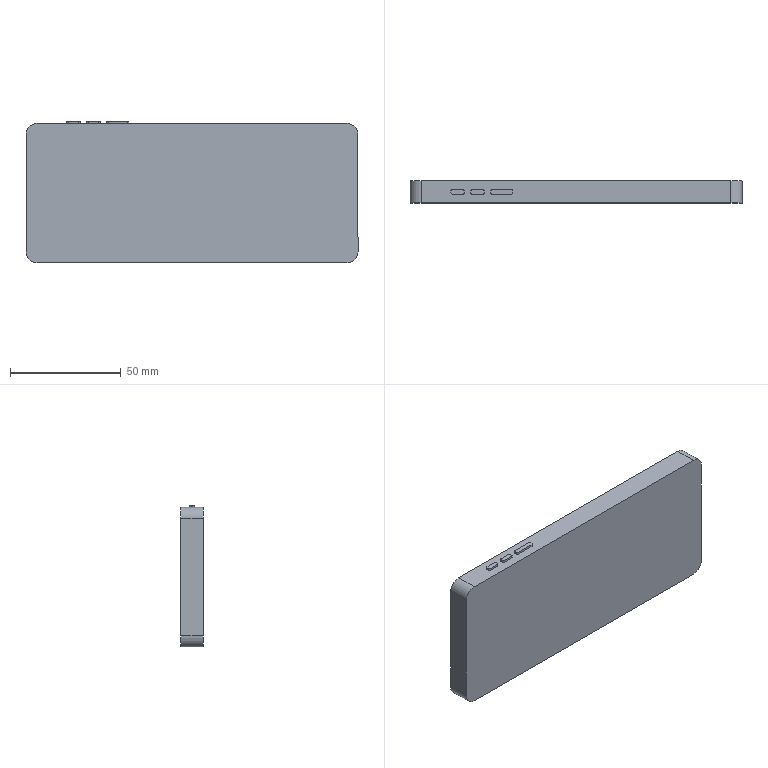Part | NX | features DATUM_CSYS 3, BLEND 2, EXTRUDE 2, SKETCH 2 | 1 solid | 37 faces | box 150 x 10 x 64.04 mm | volume 94388 mm3 | plane 21 | cylinder 16 | commonest cylinder face diameters 1.2 x12 10 x4
STEP:
#1=CARTESIAN_POINT('',(-47.486,-4.6,31.52));
#2=VERTEX_POINT('',#1);
#3=CARTESIAN_POINT('',(-47.486,-5.4,31.52));
#4=VERTEX_POINT('',#3);
#5=CARTESIAN_POINT('',(-47.486,-4.,31.52));
#6=DIRECTION('',(0.,-1.,0.));
#7=VECTOR('',#6,1000.);
#8=LINE('',#5,#7);
#9=EDGE_CURVE('',#2,#4,#8,.T.);
#10=ORIENTED_EDGE('',*,*,#9,.F.);
#11=CARTESIAN_POINT('',(-46.886,-4.,31.52));
#12=VERTEX_POINT('',#11);
#13=CARTESIAN_POINT('',(-46.886,-4.6,31.52));
#14=DIRECTION('',(0.,0.,-1.));
#15=DIRECTION('',(-1.,0.,0.));
#16=AXIS2_PLACEMENT_3D('',#13,#14,#15);
#17=CIRCLE('',#16,0.6);
#18=EDGE_CURVE('',#2,#12,#17,.T.);
#19=ORIENTED_EDGE('',*,*,#18,.T.);
#20=CARTESIAN_POINT('',(-42.086,-4.,31.52));
#21=VERTEX_POINT('',#20);
#22=CARTESIAN_POINT('',(-41.486,-4.,31.52));
#23=DIRECTION('',(-1.,0.,0.));
#24=VECTOR('',#23,1000.);
#25=LINE('',#22,#24);
#26=EDGE_CURVE('',#21,#12,#25,.T.);
#27=ORIENTED_EDGE('',*,*,#26,.F.);
#28=CARTESIAN_POINT('',(-41.486,-4.6,31.52));
#29=VERTEX_POINT('',#28);
#30=CARTESIAN_POINT('',(-42.086,-4.6,31.52));
#31=DIRECTION('',(0.,0.,-1.));
#32=DIRECTION('',(-1.,0.,0.));
#33=AXIS2_PLACEMENT_3D('',#30,#31,#32);
#34=CIRCLE('',#33,0.6);
#35=EDGE_CURVE('',#21,#29,#34,.T.);
#36=ORIENTED_EDGE('',*,*,#35,.T.);
#37=CARTESIAN_POINT('',(-41.486,-5.4,31.52));
#38=VERTEX_POINT('',#37);
#39=CARTESIAN_POINT('',(-41.486,-6.,31.52));
#40=DIRECTION('',(0.,1.,0.));
#41=VECTOR('',#40,1000.);
#42=LINE('',#39,#41);
#43=EDGE_CURVE('',#38,#29,#42,.T.);
#44=ORIENTED_EDGE('',*,*,#43,.F.);
#45=CARTESIAN_POINT('',(-42.086,-6.,31.52));
#46=VERTEX_POINT('',#45);
#47=CARTESIAN_POINT('',(-42.086,-5.4,31.52));
#48=DIRECTION('',(0.,0.,-1.));
#49=DIRECTION('',(-1.,0.,0.));
#50=AXIS2_PLACEMENT_3D('',#47,#48,#49);
#51=CIRCLE('',#50,0.6);
#52=EDGE_CURVE('',#38,#46,#51,.T.);
#53=ORIENTED_EDGE('',*,*,#52,.T.);
#54=CARTESIAN_POINT('',(-46.886,-6.,31.52));
#55=VERTEX_POINT('',#54);
#56=CARTESIAN_POINT('',(-47.486,-6.,31.52));
#57=DIRECTION('',(1.,0.,0.));
#58=VECTOR('',#57,1000.);
#59=LINE('',#56,#58);
#60=EDGE_CURVE('',#55,#46,#59,.T.);
#61=ORIENTED_EDGE('',*,*,#60,.F.);
#62=CARTESIAN_POINT('',(-46.886,-5.4,31.52));
#63=DIRECTION('',(0.,0.,-1.));
#64=DIRECTION('',(-1.,0.,0.));
#65=AXIS2_PLACEMENT_3D('',#62,#63,#64);
#66=CIRCLE('',#65,0.6);
#67=EDGE_CURVE('',#55,#4,#66,.T.);
#68=ORIENTED_EDGE('',*,*,#67,.T.);
#69=EDGE_LOOP('',(#10,#19,#27,#36,#44,#53,#61,#68));
#70=FACE_BOUND('',#69,.T.);
#71=CARTESIAN_POINT('',(70.,0.,31.52));
#72=VERTEX_POINT('',#71);
#73=CARTESIAN_POINT('',(-70.,0.,31.52));
#74=VERTEX_POINT('',#73);
#75=CARTESIAN_POINT('',(75.,0.,31.52));
#76=DIRECTION('',(-1.,0.,0.));
#77=VECTOR('',#76,1000.);
#78=LINE('',#75,#77);
#79=EDGE_CURVE('',#72,#74,#78,.T.);
#80=ORIENTED_EDGE('',*,*,#79,.T.);
#81=CARTESIAN_POINT('',(-70.,-10.,31.52));
#82=VERTEX_POINT('',#81);
#83=CARTESIAN_POINT('',(-70.,-10.,31.52));
#84=DIRECTION('',(0.,1.,0.));
#85=VECTOR('',#84,1000.);
#86=LINE('',#83,#85);
#87=EDGE_CURVE('',#74,#82,#86,.F.);
#88=ORIENTED_EDGE('',*,*,#87,.T.);
#89=CARTESIAN_POINT('',(70.,-10.,31.52));
#90=VERTEX_POINT('',#89);
#91=CARTESIAN_POINT('',(75.,-10.,31.52));
#92=DIRECTION('',(-1.,0.,0.));
#93=VECTOR('',#92,1000.);
#94=LINE('',#91,#93);
#95=EDGE_CURVE('',#90,#82,#94,.T.);
#96=ORIENTED_EDGE('',*,*,#95,.F.);
#97=CARTESIAN_POINT('',(70.,-10.,31.52));
#98=DIRECTION('',(0.,1.,0.));
#99=VECTOR('',#98,1000.);
#100=LINE('',#97,#99);
#101=EDGE_CURVE('',#90,#72,#100,.T.);
#102=ORIENTED_EDGE('',*,*,#101,.T.);
#103=EDGE_LOOP('',(#80,#88,#96,#102));
#104=FACE_BOUND('',#103,.T.);
#105=CARTESIAN_POINT('',(-38.486,-4.6,31.52));
#106=VERTEX_POINT('',#105);
#107=CARTESIAN_POINT('',(-38.486,-5.4,31.52));
#108=VERTEX_POINT('',#107);
#109=CARTESIAN_POINT('',(-38.486,-4.,31.52));
#110=DIRECTION('',(0.,-1.,0.));
#111=VECTOR('',#110,1000.);
#112=LINE('',#109,#111);
#113=EDGE_CURVE('',#106,#108,#112,.T.);
#114=ORIENTED_EDGE('',*,*,#113,.F.);
#115=CARTESIAN_POINT('',(-37.886,-4.,31.52));
#116=VERTEX_POINT('',#115);
#117=CARTESIAN_POINT('',(-37.886,-4.6,31.52));
#118=DIRECTION('',(0.,0.,-1.));
#119=DIRECTION('',(-1.,0.,0.));
#120=AXIS2_PLACEMENT_3D('',#117,#118,#119);
#121=CIRCLE('',#120,0.6);
#122=EDGE_CURVE('',#106,#116,#121,.T.);
#123=ORIENTED_EDGE('',*,*,#122,.T.);
#124=CARTESIAN_POINT('',(-29.086,-4.,31.52));
#125=VERTEX_POINT('',#124);
#126=CARTESIAN_POINT('',(-28.486,-4.,31.52));
#127=DIRECTION('',(-1.,0.,0.));
#128=VECTOR('',#127,1000.);
#129=LINE('',#126,#128);
#130=EDGE_CURVE('',#125,#116,#129,.T.);
#131=ORIENTED_EDGE('',*,*,#130,.F.);
#132=CARTESIAN_POINT('',(-28.486,-4.6,31.52));
#133=VERTEX_POINT('',#132);
#134=CARTESIAN_POINT('',(-29.086,-4.6,31.52));
#135=DIRECTION('',(0.,0.,-1.));
#136=DIRECTION('',(-1.,0.,0.));
#137=AXIS2_PLACEMENT_3D('',#134,#135,#136);
#138=CIRCLE('',#137,0.6);
#139=EDGE_CURVE('',#125,#133,#138,.T.);
#140=ORIENTED_EDGE('',*,*,#139,.T.);
#141=CARTESIAN_POINT('',(-28.486,-5.4,31.52));
#142=VERTEX_POINT('',#141);
#143=CARTESIAN_POINT('',(-28.486,-6.,31.52));
#144=DIRECTION('',(0.,1.,0.));
#145=VECTOR('',#144,1000.);
#146=LINE('',#143,#145);
#147=EDGE_CURVE('',#142,#133,#146,.T.);
#148=ORIENTED_EDGE('',*,*,#147,.F.);
#149=CARTESIAN_POINT('',(-29.086,-6.,31.52));
#150=VERTEX_POINT('',#149);
#151=CARTESIAN_POINT('',(-29.086,-5.4,31.52));
#152=DIRECTION('',(0.,0.,-1.));
#153=DIRECTION('',(-1.,0.,0.));
#154=AXIS2_PLACEMENT_3D('',#151,#152,#153);
#155=CIRCLE('',#154,0.6);
#156=EDGE_CURVE('',#142,#150,#155,.T.);
#157=ORIENTED_EDGE('',*,*,#156,.T.);
#158=CARTESIAN_POINT('',(-37.886,-6.,31.52));
#159=VERTEX_POINT('',#158);
#160=CARTESIAN_POINT('',(-38.486,-6.,31.52));
#161=DIRECTION('',(1.,0.,0.));
#162=VECTOR('',#161,1000.);
#163=LINE('',#160,#162);
#164=EDGE_CURVE('',#159,#150,#163,.T.);
#165=ORIENTED_EDGE('',*,*,#164,.F.);
#166=CARTESIAN_POINT('',(-37.886,-5.4,31.52));
#167=DIRECTION('',(0.,0.,-1.));
#168=DIRECTION('',(-1.,0.,0.));
#169=AXIS2_PLACEMENT_3D('',#166,#167,#168);
#170=CIRCLE('',#169,0.6);
#171=EDGE_CURVE('',#159,#108,#170,.T.);
#172=ORIENTED_EDGE('',*,*,#171,.T.);
#173=EDGE_LOOP('',(#114,#123,#131,#140,#148,#157,#165,#172));
#174=FACE_BOUND('',#173,.T.);
#175=CARTESIAN_POINT('',(-56.486,-4.6,31.52));
#176=VERTEX_POINT('',#175);
#177=CARTESIAN_POINT('',(-56.486,-5.4,31.52));
#178=VERTEX_POINT('',#177);
#179=CARTESIAN_POINT('',(-56.486,-4.,31.52));
#180=DIRECTION('',(0.,-1.,0.));
#181=VECTOR('',#180,1000.);
#182=LINE('',#179,#181);
#183=EDGE_CURVE('',#176,#178,#182,.T.);
#184=ORIENTED_EDGE('',*,*,#183,.F.);
#185=CARTESIAN_POINT('',(-55.886,-4.,31.52));
#186=VERTEX_POINT('',#185);
#187=CARTESIAN_POINT('',(-55.886,-4.6,31.52));
#188=DIRECTION('',(0.,0.,-1.));
#189=DIRECTION('',(-1.,0.,0.));
#190=AXIS2_PLACEMENT_3D('',#187,#188,#189);
#191=CIRCLE('',#190,0.6);
#192=EDGE_CURVE('',#176,#186,#191,.T.);
#193=ORIENTED_EDGE('',*,*,#192,.T.);
#194=CARTESIAN_POINT('',(-51.086,-4.,31.52));
#195=VERTEX_POINT('',#194);
#196=CARTESIAN_POINT('',(-50.486,-4.,31.52));
#197=DIRECTION('',(-1.,0.,0.));
#198=VECTOR('',#197,1000.);
#199=LINE('',#196,#198);
#200=EDGE_CURVE('',#195,#186,#199,.T.);
#201=ORIENTED_EDGE('',*,*,#200,.F.);
#202=CARTESIAN_POINT('',(-50.486,-4.6,31.52));
#203=VERTEX_POINT('',#202);
#204=CARTESIAN_POINT('',(-51.086,-4.6,31.52));
#205=DIRECTION('',(0.,0.,-1.));
#206=DIRECTION('',(-1.,0.,0.));
#207=AXIS2_PLACEMENT_3D('',#204,#205,#206);
#208=CIRCLE('',#207,0.6);
#209=EDGE_CURVE('',#195,#203,#208,.T.);
#210=ORIENTED_EDGE('',*,*,#209,.T.);
#211=CARTESIAN_POINT('',(-50.486,-5.4,31.52));
#212=VERTEX_POINT('',#211);
#213=CARTESIAN_POINT('',(-50.486,-6.,31.52));
#214=DIRECTION('',(0.,1.,0.));
#215=VECTOR('',#214,1000.);
#216=LINE('',#213,#215);
#217=EDGE_CURVE('',#212,#203,#216,.T.);
#218=ORIENTED_EDGE('',*,*,#217,.F.);
#219=CARTESIAN_POINT('',(-51.086,-6.,31.52));
#220=VERTEX_POINT('',#219);
#221=CARTESIAN_POINT('',(-51.086,-5.4,31.52));
#222=DIRECTION('',(0.,0.,-1.));
#223=DIRECTION('',(-1.,0.,0.));
#224=AXIS2_PLACEMENT_3D('',#221,#222,#223);
#225=CIRCLE('',#224,0.6);
#226=EDGE_CURVE('',#212,#220,#225,.T.);
#227=ORIENTED_EDGE('',*,*,#226,.T.);
#228=CARTESIAN_POINT('',(-55.886,-6.,31.52));
#229=VERTEX_POINT('',#228);
#230=CARTESIAN_POINT('',(-56.486,-6.,31.52));
#231=DIRECTION('',(1.,0.,0.));
#232=VECTOR('',#231,1000.);
#233=LINE('',#230,#232);
#234=EDGE_CURVE('',#229,#220,#233,.T.);
#235=ORIENTED_EDGE('',*,*,#234,.F.);
#236=CARTESIAN_POINT('',(-55.886,-5.4,31.52));
#237=DIRECTION('',(0.,0.,-1.));
#238=DIRECTION('',(-1.,0.,0.));
#239=AXIS2_PLACEMENT_3D('',#236,#237,#238);
#240=CIRCLE('',#239,0.6);
#241=EDGE_CURVE('',#229,#178,#240,.T.);
#242=ORIENTED_EDGE('',*,*,#241,.T.);
#243=EDGE_LOOP('',(#184,#193,#201,#210,#218,#227,#235,#242));
#244=FACE_BOUND('',#243,.T.);
#245=CARTESIAN_POINT('',(75.,-10.,31.52));
#246=DIRECTION('',(0.,0.,-1.));
#247=DIRECTION('',(-1.,0.,0.));
#248=AXIS2_PLACEMENT_3D('',#245,#246,#247);
#249=PLANE('',#248);
#250=ADVANCED_FACE('',(#70,#104,#174,#244),#249,.F.);
#251=CARTESIAN_POINT('',(-75.,-10.,26.52));
#252=VERTEX_POINT('',#251);
#253=CARTESIAN_POINT('',(-75.,-10.,-26.52));
#254=VERTEX_POINT('',#253);
#255=CARTESIAN_POINT('',(-75.,-10.,31.52));
#256=DIRECTION('',(0.,0.,-1.));
#257=VECTOR('',#256,1000.);
#258=LINE('',#255,#257);
#259=EDGE_CURVE('',#252,#254,#258,.T.);
#260=ORIENTED_EDGE('',*,*,#259,.F.);
#261=CARTESIAN_POINT('',(-75.,0.,26.52));
#262=VERTEX_POINT('',#261);
#263=CARTESIAN_POINT('',(-75.,-10.,26.52));
#264=DIRECTION('',(0.,1.,0.));
#265=VECTOR('',#264,1000.);
#266=LINE('',#263,#265);
#267=EDGE_CURVE('',#252,#262,#266,.T.);
#268=ORIENTED_EDGE('',*,*,#267,.T.);
#269=CARTESIAN_POINT('',(-75.,0.,-26.52));
#270=VERTEX_POINT('',#269);
#271=CARTESIAN_POINT('',(-75.,0.,31.52));
#272=DIRECTION('',(0.,0.,-1.));
#273=VECTOR('',#272,1000.);
#274=LINE('',#271,#273);
#275=EDGE_CURVE('',#262,#270,#274,.T.);
#276=ORIENTED_EDGE('',*,*,#275,.T.);
#277=CARTESIAN_POINT('',(-75.,-10.,-26.52));
#278=DIRECTION('',(0.,1.,0.));
#279=VECTOR('',#278,1000.);
#280=LINE('',#277,#279);
#281=EDGE_CURVE('',#270,#254,#280,.F.);
#282=ORIENTED_EDGE('',*,*,#281,.T.);
#283=EDGE_LOOP('',(#260,#268,#276,#282));
#284=FACE_BOUND('',#283,.T.);
#285=CARTESIAN_POINT('',(-75.,-10.,31.52));
#286=DIRECTION('',(1.,0.,0.));
#287=DIRECTION('',(0.,0.,-1.));
#288=AXIS2_PLACEMENT_3D('',#285,#286,#287);
#289=PLANE('',#288);
#290=ADVANCED_FACE('',(#284),#289,.F.);
#291=CARTESIAN_POINT('',(-70.,-10.,-31.52));
#292=VERTEX_POINT('',#291);
#293=CARTESIAN_POINT('',(70.,-10.,-31.52));
#294=VERTEX_POINT('',#293);
#295=CARTESIAN_POINT('',(-75.,-10.,-31.52));
#296=DIRECTION('',(1.,0.,0.));
#297=VECTOR('',#296,1000.);
#298=LINE('',#295,#297);
#299=EDGE_CURVE('',#292,#294,#298,.T.);
#300=ORIENTED_EDGE('',*,*,#299,.F.);
#301=CARTESIAN_POINT('',(-70.,0.,-31.52));
#302=VERTEX_POINT('',#301);
#303=CARTESIAN_POINT('',(-70.,-10.,-31.52));
#304=DIRECTION('',(0.,1.,0.));
#305=VECTOR('',#304,1000.);
#306=LINE('',#303,#305);
#307=EDGE_CURVE('',#292,#302,#306,.T.);
#308=ORIENTED_EDGE('',*,*,#307,.T.);
#309=CARTESIAN_POINT('',(70.,0.,-31.52));
#310=VERTEX_POINT('',#309);
#311=CARTESIAN_POINT('',(-75.,0.,-31.52));
#312=DIRECTION('',(1.,0.,0.));
#313=VECTOR('',#312,1000.);
#314=LINE('',#311,#313);
#315=EDGE_CURVE('',#302,#310,#314,.T.);
#316=ORIENTED_EDGE('',*,*,#315,.T.);
#317=CARTESIAN_POINT('',(70.,-10.,-31.52));
#318=DIRECTION('',(0.,1.,0.));
#319=VECTOR('',#318,1000.);
#320=LINE('',#317,#319);
#321=EDGE_CURVE('',#310,#294,#320,.F.);
#322=ORIENTED_EDGE('',*,*,#321,.T.);
#323=EDGE_LOOP('',(#300,#308,#316,#322));
#324=FACE_BOUND('',#323,.T.);
#325=CARTESIAN_POINT('',(-75.,-10.,-31.52));
#326=DIRECTION('',(0.,0.,1.));
#327=DIRECTION('',(1.,0.,0.));
#328=AXIS2_PLACEMENT_3D('',#325,#326,#327);
#329=PLANE('',#328);
#330=ADVANCED_FACE('',(#324),#329,.F.);
#331=CARTESIAN_POINT('',(75.,-10.,-26.52));
#332=VERTEX_POINT('',#331);
#333=CARTESIAN_POINT('',(75.,-10.,26.52));
#334=VERTEX_POINT('',#333);
#335=CARTESIAN_POINT('',(75.,-10.,-31.52));
#336=DIRECTION('',(0.,0.,1.));
#337=VECTOR('',#336,1000.);
#338=LINE('',#335,#337);
#339=EDGE_CURVE('',#332,#334,#338,.T.);
#340=ORIENTED_EDGE('',*,*,#339,.F.);
#341=CARTESIAN_POINT('',(75.,0.,-26.52));
#342=VERTEX_POINT('',#341);
#343=CARTESIAN_POINT('',(75.,-10.,-26.52));
#344=DIRECTION('',(0.,1.,0.));
#345=VECTOR('',#344,1000.);
#346=LINE('',#343,#345);
#347=EDGE_CURVE('',#332,#342,#346,.T.);
#348=ORIENTED_EDGE('',*,*,#347,.T.);
#349=CARTESIAN_POINT('',(75.,0.,26.52));
#350=VERTEX_POINT('',#349);
#351=CARTESIAN_POINT('',(75.,0.,-31.52));
#352=DIRECTION('',(0.,0.,1.));
#353=VECTOR('',#352,1000.);
#354=LINE('',#351,#353);
#355=EDGE_CURVE('',#342,#350,#354,.T.);
#356=ORIENTED_EDGE('',*,*,#355,.T.);
#357=CARTESIAN_POINT('',(75.,-10.,26.52));
#358=DIRECTION('',(0.,1.,0.));
#359=VECTOR('',#358,1000.);
#360=LINE('',#357,#359);
#361=EDGE_CURVE('',#350,#334,#360,.F.);
#362=ORIENTED_EDGE('',*,*,#361,.T.);
#363=EDGE_LOOP('',(#340,#348,#356,#362));
#364=FACE_BOUND('',#363,.T.);
#365=CARTESIAN_POINT('',(75.,-10.,-31.52));
#366=DIRECTION('',(-1.,0.,0.));
#367=DIRECTION('',(0.,0.,1.));
#368=AXIS2_PLACEMENT_3D('',#365,#366,#367);
#369=PLANE('',#368);
#370=ADVANCED_FACE('',(#364),#369,.F.);
#371=ORIENTED_EDGE('',*,*,#95,.T.);
#372=CARTESIAN_POINT('',(-70.,-10.,26.52));
#373=DIRECTION('',(0.,-1.,0.));
#374=DIRECTION('',(0.,0.,-1.));
#375=AXIS2_PLACEMENT_3D('',#372,#373,#374);
#376=CIRCLE('',#375,5.);
#377=EDGE_CURVE('',#82,#252,#376,.T.);
#378=ORIENTED_EDGE('',*,*,#377,.T.);
#379=ORIENTED_EDGE('',*,*,#259,.T.);
#380=CARTESIAN_POINT('',(-70.,-10.,-26.52));
#381=DIRECTION('',(0.,-1.,0.));
#382=DIRECTION('',(0.,0.,-1.));
#383=AXIS2_PLACEMENT_3D('',#380,#381,#382);
#384=CIRCLE('',#383,5.);
#385=EDGE_CURVE('',#254,#292,#384,.T.);
#386=ORIENTED_EDGE('',*,*,#385,.T.);
#387=ORIENTED_EDGE('',*,*,#299,.T.);
#388=CARTESIAN_POINT('',(70.,-10.,-26.52));
#389=DIRECTION('',(0.,-1.,0.));
#390=DIRECTION('',(0.,0.,-1.));
#391=AXIS2_PLACEMENT_3D('',#388,#389,#390);
#392=CIRCLE('',#391,5.);
#393=EDGE_CURVE('',#294,#332,#392,.T.);
#394=ORIENTED_EDGE('',*,*,#393,.T.);
#395=ORIENTED_EDGE('',*,*,#339,.T.);
#396=CARTESIAN_POINT('',(70.,-10.,26.52));
#397=DIRECTION('',(0.,-1.,0.));
#398=DIRECTION('',(0.,0.,-1.));
#399=AXIS2_PLACEMENT_3D('',#396,#397,#398);
#400=CIRCLE('',#399,5.);
#401=EDGE_CURVE('',#334,#90,#400,.T.);
#402=ORIENTED_EDGE('',*,*,#401,.T.);
#403=EDGE_LOOP('',(#371,#378,#379,#386,#387,#394,#395,#402));
#404=FACE_BOUND('',#403,.T.);
#405=CARTESIAN_POINT('',(0.,-10.,0.));
#406=DIRECTION('',(0.,-1.,0.));
#407=DIRECTION('',(0.,0.,-1.));
#408=AXIS2_PLACEMENT_3D('',#405,#406,#407);
#409=PLANE('',#408);
#410=ADVANCED_FACE('',(#404),#409,.T.);
#411=ORIENTED_EDGE('',*,*,#275,.F.);
#412=CARTESIAN_POINT('',(-70.,0.,26.52));
#413=DIRECTION('',(0.,-1.,0.));
#414=DIRECTION('',(0.,0.,-1.));
#415=AXIS2_PLACEMENT_3D('',#412,#413,#414);
#416=CIRCLE('',#415,5.);
#417=EDGE_CURVE('',#262,#74,#416,.F.);
#418=ORIENTED_EDGE('',*,*,#417,.T.);
#419=ORIENTED_EDGE('',*,*,#79,.F.);
#420=CARTESIAN_POINT('',(70.,0.,26.52));
#421=DIRECTION('',(0.,-1.,0.));
#422=DIRECTION('',(0.,0.,-1.));
#423=AXIS2_PLACEMENT_3D('',#420,#421,#422);
#424=CIRCLE('',#423,5.);
#425=EDGE_CURVE('',#72,#350,#424,.F.);
#426=ORIENTED_EDGE('',*,*,#425,.T.);
#427=ORIENTED_EDGE('',*,*,#355,.F.);
#428=CARTESIAN_POINT('',(70.,0.,-26.52));
#429=DIRECTION('',(0.,-1.,0.));
#430=DIRECTION('',(0.,0.,-1.));
#431=AXIS2_PLACEMENT_3D('',#428,#429,#430);
#432=CIRCLE('',#431,5.);
#433=EDGE_CURVE('',#342,#310,#432,.F.);
#434=ORIENTED_EDGE('',*,*,#433,.T.);
#435=ORIENTED_EDGE('',*,*,#315,.F.);
#436=CARTESIAN_POINT('',(-70.,0.,-26.52));
#437=DIRECTION('',(0.,-1.,0.));
#438=DIRECTION('',(0.,0.,-1.));
#439=AXIS2_PLACEMENT_3D('',#436,#437,#438);
#440=CIRCLE('',#439,5.);
#441=EDGE_CURVE('',#302,#270,#440,.F.);
#442=ORIENTED_EDGE('',*,*,#441,.T.);
#443=EDGE_LOOP('',(#411,#418,#419,#426,#427,#434,#435,#442));
#444=FACE_BOUND('',#443,.T.);
#445=CARTESIAN_POINT('',(0.,0.,0.));
#446=DIRECTION('',(0.,-1.,0.));
#447=DIRECTION('',(0.,0.,-1.));
#448=AXIS2_PLACEMENT_3D('',#445,#446,#447);
#449=PLANE('',#448);
#450=ADVANCED_FACE('',(#444),#449,.F.);
#451=ORIENTED_EDGE('',*,*,#377,.F.);
#452=ORIENTED_EDGE('',*,*,#87,.F.);
#453=ORIENTED_EDGE('',*,*,#417,.F.);
#454=ORIENTED_EDGE('',*,*,#267,.F.);
#455=EDGE_LOOP('',(#451,#452,#453,#454));
#456=FACE_BOUND('',#455,.T.);
#457=CARTESIAN_POINT('',(-70.,-10.,26.52));
#458=DIRECTION('',(0.,1.,0.));
#459=DIRECTION('',(0.,0.,1.));
#460=AXIS2_PLACEMENT_3D('',#457,#458,#459);
#461=CYLINDRICAL_SURFACE('',#460,5.);
#462=ADVANCED_FACE('',(#456),#461,.T.);
#463=ORIENTED_EDGE('',*,*,#385,.F.);
#464=ORIENTED_EDGE('',*,*,#281,.F.);
#465=ORIENTED_EDGE('',*,*,#441,.F.);
#466=ORIENTED_EDGE('',*,*,#307,.F.);
#467=EDGE_LOOP('',(#463,#464,#465,#466));
#468=FACE_BOUND('',#467,.T.);
#469=CARTESIAN_POINT('',(-70.,-10.,-26.52));
#470=DIRECTION('',(0.,1.,0.));
#471=DIRECTION('',(0.,0.,1.));
#472=AXIS2_PLACEMENT_3D('',#469,#470,#471);
#473=CYLINDRICAL_SURFACE('',#472,5.);
#474=ADVANCED_FACE('',(#468),#473,.T.);
#475=ORIENTED_EDGE('',*,*,#393,.F.);
#476=ORIENTED_EDGE('',*,*,#321,.F.);
#477=ORIENTED_EDGE('',*,*,#433,.F.);
#478=ORIENTED_EDGE('',*,*,#347,.F.);
#479=EDGE_LOOP('',(#475,#476,#477,#478));
#480=FACE_BOUND('',#479,.T.);
#481=CARTESIAN_POINT('',(70.,-10.,-26.52));
#482=DIRECTION('',(0.,1.,0.));
#483=DIRECTION('',(0.,0.,1.));
#484=AXIS2_PLACEMENT_3D('',#481,#482,#483);
#485=CYLINDRICAL_SURFACE('',#484,5.);
#486=ADVANCED_FACE('',(#480),#485,.T.);
#487=ORIENTED_EDGE('',*,*,#401,.F.);
#488=ORIENTED_EDGE('',*,*,#361,.F.);
#489=ORIENTED_EDGE('',*,*,#425,.F.);
#490=ORIENTED_EDGE('',*,*,#101,.F.);
#491=EDGE_LOOP('',(#487,#488,#489,#490));
#492=FACE_BOUND('',#491,.T.);
#493=CARTESIAN_POINT('',(70.,-10.,26.52));
#494=DIRECTION('',(0.,1.,0.));
#495=DIRECTION('',(0.,0.,1.));
#496=AXIS2_PLACEMENT_3D('',#493,#494,#495);
#497=CYLINDRICAL_SURFACE('',#496,5.);
#498=ADVANCED_FACE('',(#492),#497,.T.);
#499=ORIENTED_EDGE('',*,*,#113,.T.);
#500=CARTESIAN_POINT('',(-38.486,-5.4,32.52));
#501=VERTEX_POINT('',#500);
#502=CARTESIAN_POINT('',(-38.486,-5.4,32.52));
#503=DIRECTION('',(0.,0.,-1.));
#504=VECTOR('',#503,1000.);
#505=LINE('',#502,#504);
#506=EDGE_CURVE('',#108,#501,#505,.F.);
#507=ORIENTED_EDGE('',*,*,#506,.T.);
#508=CARTESIAN_POINT('',(-38.486,-4.6,32.52));
#509=VERTEX_POINT('',#508);
#510=CARTESIAN_POINT('',(-38.486,-4.,32.52));
#511=DIRECTION('',(0.,-1.,0.));
#512=VECTOR('',#511,1000.);
#513=LINE('',#510,#512);
#514=EDGE_CURVE('',#509,#501,#513,.T.);
#515=ORIENTED_EDGE('',*,*,#514,.F.);
#516=CARTESIAN_POINT('',(-38.486,-4.6,32.52));
#517=DIRECTION('',(0.,0.,-1.));
#518=VECTOR('',#517,1000.);
#519=LINE('',#516,#518);
#520=EDGE_CURVE('',#509,#106,#519,.T.);
#521=ORIENTED_EDGE('',*,*,#520,.T.);
#522=EDGE_LOOP('',(#499,#507,#515,#521));
#523=FACE_BOUND('',#522,.T.);
#524=CARTESIAN_POINT('',(-38.486,-4.,32.52));
#525=DIRECTION('',(1.,0.,0.));
#526=DIRECTION('',(0.,0.,-1.));
#527=AXIS2_PLACEMENT_3D('',#524,#525,#526);
#528=PLANE('',#527);
#529=ADVANCED_FACE('',(#523),#528,.F.);
#530=CARTESIAN_POINT('',(-37.886,-6.,32.52));
#531=VERTEX_POINT('',#530);
#532=CARTESIAN_POINT('',(-29.086,-6.,32.52));
#533=VERTEX_POINT('',#532);
#534=CARTESIAN_POINT('',(-38.486,-6.,32.52));
#535=DIRECTION('',(1.,0.,0.));
#536=VECTOR('',#535,1000.);
#537=LINE('',#534,#536);
#538=EDGE_CURVE('',#531,#533,#537,.T.);
#539=ORIENTED_EDGE('',*,*,#538,.F.);
#540=CARTESIAN_POINT('',(-37.886,-6.,32.52));
#541=DIRECTION('',(0.,0.,-1.));
#542=VECTOR('',#541,1000.);
#543=LINE('',#540,#542);
#544=EDGE_CURVE('',#531,#159,#543,.T.);
#545=ORIENTED_EDGE('',*,*,#544,.T.);
#546=ORIENTED_EDGE('',*,*,#164,.T.);
#547=CARTESIAN_POINT('',(-29.086,-6.,32.52));
#548=DIRECTION('',(0.,0.,-1.));
#549=VECTOR('',#548,1000.);
#550=LINE('',#547,#549);
#551=EDGE_CURVE('',#150,#533,#550,.F.);
#552=ORIENTED_EDGE('',*,*,#551,.T.);
#553=EDGE_LOOP('',(#539,#545,#546,#552));
#554=FACE_BOUND('',#553,.T.);
#555=CARTESIAN_POINT('',(-38.486,-6.,32.52));
#556=DIRECTION('',(0.,1.,0.));
#557=DIRECTION('',(0.,0.,1.));
#558=AXIS2_PLACEMENT_3D('',#555,#556,#557);
#559=PLANE('',#558);
#560=ADVANCED_FACE('',(#554),#559,.F.);
#561=CARTESIAN_POINT('',(-28.486,-5.4,32.52));
#562=VERTEX_POINT('',#561);
#563=CARTESIAN_POINT('',(-28.486,-4.6,32.52));
#564=VERTEX_POINT('',#563);
#565=CARTESIAN_POINT('',(-28.486,-6.,32.52));
#566=DIRECTION('',(0.,1.,0.));
#567=VECTOR('',#566,1000.);
#568=LINE('',#565,#567);
#569=EDGE_CURVE('',#562,#564,#568,.T.);
#570=ORIENTED_EDGE('',*,*,#569,.F.);
#571=CARTESIAN_POINT('',(-28.486,-5.4,32.52));
#572=DIRECTION('',(0.,0.,-1.));
#573=VECTOR('',#572,1000.);
#574=LINE('',#571,#573);
#575=EDGE_CURVE('',#562,#142,#574,.T.);
#576=ORIENTED_EDGE('',*,*,#575,.T.);
#577=ORIENTED_EDGE('',*,*,#147,.T.);
#578=CARTESIAN_POINT('',(-28.486,-4.6,32.52));
#579=DIRECTION('',(0.,0.,-1.));
#580=VECTOR('',#579,1000.);
#581=LINE('',#578,#580);
#582=EDGE_CURVE('',#133,#564,#581,.F.);
#583=ORIENTED_EDGE('',*,*,#582,.T.);
#584=EDGE_LOOP('',(#570,#576,#577,#583));
#585=FACE_BOUND('',#584,.T.);
#586=CARTESIAN_POINT('',(-28.486,-6.,32.52));
#587=DIRECTION('',(-1.,0.,0.));
#588=DIRECTION('',(0.,0.,1.));
#589=AXIS2_PLACEMENT_3D('',#586,#587,#588);
#590=PLANE('',#589);
#591=ADVANCED_FACE('',(#585),#590,.F.);
#592=ORIENTED_EDGE('',*,*,#130,.T.);
#593=CARTESIAN_POINT('',(-37.886,-4.,32.52));
#594=VERTEX_POINT('',#593);
#595=CARTESIAN_POINT('',(-37.886,-4.,32.52));
#596=DIRECTION('',(0.,0.,-1.));
#597=VECTOR('',#596,1000.);
#598=LINE('',#595,#597);
#599=EDGE_CURVE('',#116,#594,#598,.F.);
#600=ORIENTED_EDGE('',*,*,#599,.T.);
#601=CARTESIAN_POINT('',(-29.086,-4.,32.52));
#602=VERTEX_POINT('',#601);
#603=CARTESIAN_POINT('',(-28.486,-4.,32.52));
#604=DIRECTION('',(-1.,0.,0.));
#605=VECTOR('',#604,1000.);
#606=LINE('',#603,#605);
#607=EDGE_CURVE('',#602,#594,#606,.T.);
#608=ORIENTED_EDGE('',*,*,#607,.F.);
#609=CARTESIAN_POINT('',(-29.086,-4.,32.52));
#610=DIRECTION('',(0.,0.,-1.));
#611=VECTOR('',#610,1000.);
#612=LINE('',#609,#611);
#613=EDGE_CURVE('',#602,#125,#612,.T.);
#614=ORIENTED_EDGE('',*,*,#613,.T.);
#615=EDGE_LOOP('',(#592,#600,#608,#614));
#616=FACE_BOUND('',#615,.T.);
#617=CARTESIAN_POINT('',(-28.486,-4.,32.52));
#618=DIRECTION('',(0.,-1.,0.));
#619=DIRECTION('',(1.,0.,0.));
#620=AXIS2_PLACEMENT_3D('',#617,#618,#619);
#621=PLANE('',#620);
#622=ADVANCED_FACE('',(#616),#621,.F.);
#623=ORIENTED_EDGE('',*,*,#514,.T.);
#624=CARTESIAN_POINT('',(-37.886,-5.4,32.52));
#625=DIRECTION('',(0.,0.,1.));
#626=DIRECTION('',(1.,0.,0.));
#627=AXIS2_PLACEMENT_3D('',#624,#625,#626);
#628=CIRCLE('',#627,0.6);
#629=EDGE_CURVE('',#501,#531,#628,.T.);
#630=ORIENTED_EDGE('',*,*,#629,.T.);
#631=ORIENTED_EDGE('',*,*,#538,.T.);
#632=CARTESIAN_POINT('',(-29.086,-5.4,32.52));
#633=DIRECTION('',(0.,0.,1.));
#634=DIRECTION('',(1.,0.,0.));
#635=AXIS2_PLACEMENT_3D('',#632,#633,#634);
#636=CIRCLE('',#635,0.6);
#637=EDGE_CURVE('',#533,#562,#636,.T.);
#638=ORIENTED_EDGE('',*,*,#637,.T.);
#639=ORIENTED_EDGE('',*,*,#569,.T.);
#640=CARTESIAN_POINT('',(-29.086,-4.6,32.52));
#641=DIRECTION('',(0.,0.,1.));
#642=DIRECTION('',(1.,0.,0.));
#643=AXIS2_PLACEMENT_3D('',#640,#641,#642);
#644=CIRCLE('',#643,0.6);
#645=EDGE_CURVE('',#564,#602,#644,.T.);
#646=ORIENTED_EDGE('',*,*,#645,.T.);
#647=ORIENTED_EDGE('',*,*,#607,.T.);
#648=CARTESIAN_POINT('',(-37.886,-4.6,32.52));
#649=DIRECTION('',(0.,0.,1.));
#650=DIRECTION('',(1.,0.,0.));
#651=AXIS2_PLACEMENT_3D('',#648,#649,#650);
#652=CIRCLE('',#651,0.6);
#653=EDGE_CURVE('',#594,#509,#652,.T.);
#654=ORIENTED_EDGE('',*,*,#653,.T.);
#655=EDGE_LOOP('',(#623,#630,#631,#638,#639,#646,#647,#654));
#656=FACE_BOUND('',#655,.T.);
#657=CARTESIAN_POINT('',(0.,0.,32.52));
#658=DIRECTION('',(0.,0.,1.));
#659=DIRECTION('',(1.,0.,0.));
#660=AXIS2_PLACEMENT_3D('',#657,#658,#659);
#661=PLANE('',#660);
#662=ADVANCED_FACE('',(#656),#661,.T.);
#663=CARTESIAN_POINT('',(-47.486,-4.6,32.52));
#664=VERTEX_POINT('',#663);
#665=CARTESIAN_POINT('',(-47.486,-5.4,32.52));
#666=VERTEX_POINT('',#665);
#667=CARTESIAN_POINT('',(-47.486,-4.,32.52));
#668=DIRECTION('',(0.,-1.,0.));
#669=VECTOR('',#668,1000.);
#670=LINE('',#667,#669);
#671=EDGE_CURVE('',#664,#666,#670,.T.);
#672=ORIENTED_EDGE('',*,*,#671,.F.);
#673=CARTESIAN_POINT('',(-47.486,-4.6,32.52));
#674=DIRECTION('',(0.,0.,-1.));
#675=VECTOR('',#674,1000.);
#676=LINE('',#673,#675);
#677=EDGE_CURVE('',#664,#2,#676,.T.);
#678=ORIENTED_EDGE('',*,*,#677,.T.);
#679=ORIENTED_EDGE('',*,*,#9,.T.);
#680=CARTESIAN_POINT('',(-47.486,-5.4,32.52));
#681=DIRECTION('',(0.,0.,-1.));
#682=VECTOR('',#681,1000.);
#683=LINE('',#680,#682);
#684=EDGE_CURVE('',#4,#666,#683,.F.);
#685=ORIENTED_EDGE('',*,*,#684,.T.);
#686=EDGE_LOOP('',(#672,#678,#679,#685));
#687=FACE_BOUND('',#686,.T.);
#688=CARTESIAN_POINT('',(-47.486,-4.,32.52));
#689=DIRECTION('',(1.,0.,0.));
#690=DIRECTION('',(0.,0.,-1.));
#691=AXIS2_PLACEMENT_3D('',#688,#689,#690);
#692=PLANE('',#691);
#693=ADVANCED_FACE('',(#687),#692,.F.);
#694=CARTESIAN_POINT('',(-46.886,-6.,32.52));
#695=VERTEX_POINT('',#694);
#696=CARTESIAN_POINT('',(-42.086,-6.,32.52));
#697=VERTEX_POINT('',#696);
#698=CARTESIAN_POINT('',(-47.486,-6.,32.52));
#699=DIRECTION('',(1.,0.,0.));
#700=VECTOR('',#699,1000.);
#701=LINE('',#698,#700);
#702=EDGE_CURVE('',#695,#697,#701,.T.);
#703=ORIENTED_EDGE('',*,*,#702,.F.);
#704=CARTESIAN_POINT('',(-46.886,-6.,32.52));
#705=DIRECTION('',(0.,0.,-1.));
#706=VECTOR('',#705,1000.);
#707=LINE('',#704,#706);
#708=EDGE_CURVE('',#695,#55,#707,.T.);
#709=ORIENTED_EDGE('',*,*,#708,.T.);
#710=ORIENTED_EDGE('',*,*,#60,.T.);
#711=CARTESIAN_POINT('',(-42.086,-6.,32.52));
#712=DIRECTION('',(0.,0.,-1.));
#713=VECTOR('',#712,1000.);
#714=LINE('',#711,#713);
#715=EDGE_CURVE('',#46,#697,#714,.F.);
#716=ORIENTED_EDGE('',*,*,#715,.T.);
#717=EDGE_LOOP('',(#703,#709,#710,#716));
#718=FACE_BOUND('',#717,.T.);
#719=CARTESIAN_POINT('',(-47.486,-6.,32.52));
#720=DIRECTION('',(0.,1.,0.));
#721=DIRECTION('',(-1.,0.,0.));
#722=AXIS2_PLACEMENT_3D('',#719,#720,#721);
#723=PLANE('',#722);
#724=ADVANCED_FACE('',(#718),#723,.F.);
#725=CARTESIAN_POINT('',(-41.486,-5.4,32.52));
#726=VERTEX_POINT('',#725);
#727=CARTESIAN_POINT('',(-41.486,-4.6,32.52));
#728=VERTEX_POINT('',#727);
#729=CARTESIAN_POINT('',(-41.486,-6.,32.52));
#730=DIRECTION('',(0.,1.,0.));
#731=VECTOR('',#730,1000.);
#732=LINE('',#729,#731);
#733=EDGE_CURVE('',#726,#728,#732,.T.);
#734=ORIENTED_EDGE('',*,*,#733,.F.);
#735=CARTESIAN_POINT('',(-41.486,-5.4,32.52));
#736=DIRECTION('',(0.,0.,-1.));
#737=VECTOR('',#736,1000.);
#738=LINE('',#735,#737);
#739=EDGE_CURVE('',#726,#38,#738,.T.);
#740=ORIENTED_EDGE('',*,*,#739,.T.);
#741=ORIENTED_EDGE('',*,*,#43,.T.);
#742=CARTESIAN_POINT('',(-41.486,-4.6,32.52));
#743=DIRECTION('',(0.,0.,-1.));
#744=VECTOR('',#743,1000.);
#745=LINE('',#742,#744);
#746=EDGE_CURVE('',#29,#728,#745,.F.);
#747=ORIENTED_EDGE('',*,*,#746,.T.);
#748=EDGE_LOOP('',(#734,#740,#741,#747));
#749=FACE_BOUND('',#748,.T.);
#750=CARTESIAN_POINT('',(-41.486,-6.,32.52));
#751=DIRECTION('',(-1.,0.,0.));
#752=DIRECTION('',(0.,0.,1.));
#753=AXIS2_PLACEMENT_3D('',#750,#751,#752);
#754=PLANE('',#753);
#755=ADVANCED_FACE('',(#749),#754,.F.);
#756=ORIENTED_EDGE('',*,*,#26,.T.);
#757=CARTESIAN_POINT('',(-46.886,-4.,32.52));
#758=VERTEX_POINT('',#757);
#759=CARTESIAN_POINT('',(-46.886,-4.,32.52));
#760=DIRECTION('',(0.,0.,-1.));
#761=VECTOR('',#760,1000.);
#762=LINE('',#759,#761);
#763=EDGE_CURVE('',#12,#758,#762,.F.);
#764=ORIENTED_EDGE('',*,*,#763,.T.);
#765=CARTESIAN_POINT('',(-42.086,-4.,32.52));
#766=VERTEX_POINT('',#765);
#767=CARTESIAN_POINT('',(-41.486,-4.,32.52));
#768=DIRECTION('',(-1.,0.,0.));
#769=VECTOR('',#768,1000.);
#770=LINE('',#767,#769);
#771=EDGE_CURVE('',#766,#758,#770,.T.);
#772=ORIENTED_EDGE('',*,*,#771,.F.);
#773=CARTESIAN_POINT('',(-42.086,-4.,32.52));
#774=DIRECTION('',(0.,0.,-1.));
#775=VECTOR('',#774,1000.);
#776=LINE('',#773,#775);
#777=EDGE_CURVE('',#766,#21,#776,.T.);
#778=ORIENTED_EDGE('',*,*,#777,.T.);
#779=EDGE_LOOP('',(#756,#764,#772,#778));
#780=FACE_BOUND('',#779,.T.);
#781=CARTESIAN_POINT('',(-41.486,-4.,32.52));
#782=DIRECTION('',(0.,-1.,0.));
#783=DIRECTION('',(0.,0.,-1.));
#784=AXIS2_PLACEMENT_3D('',#781,#782,#783);
#785=PLANE('',#784);
#786=ADVANCED_FACE('',(#780),#785,.F.);
#787=ORIENTED_EDGE('',*,*,#771,.T.);
#788=CARTESIAN_POINT('',(-46.886,-4.6,32.52));
#789=DIRECTION('',(0.,0.,1.));
#790=DIRECTION('',(1.,0.,0.));
#791=AXIS2_PLACEMENT_3D('',#788,#789,#790);
#792=CIRCLE('',#791,0.6);
#793=EDGE_CURVE('',#758,#664,#792,.T.);
#794=ORIENTED_EDGE('',*,*,#793,.T.);
#795=ORIENTED_EDGE('',*,*,#671,.T.);
#796=CARTESIAN_POINT('',(-46.886,-5.4,32.52));
#797=DIRECTION('',(0.,0.,1.));
#798=DIRECTION('',(1.,0.,0.));
#799=AXIS2_PLACEMENT_3D('',#796,#797,#798);
#800=CIRCLE('',#799,0.6);
#801=EDGE_CURVE('',#666,#695,#800,.T.);
#802=ORIENTED_EDGE('',*,*,#801,.T.);
#803=ORIENTED_EDGE('',*,*,#702,.T.);
#804=CARTESIAN_POINT('',(-42.086,-5.4,32.52));
#805=DIRECTION('',(0.,0.,1.));
#806=DIRECTION('',(1.,0.,0.));
#807=AXIS2_PLACEMENT_3D('',#804,#805,#806);
#808=CIRCLE('',#807,0.6);
#809=EDGE_CURVE('',#697,#726,#808,.T.);
#810=ORIENTED_EDGE('',*,*,#809,.T.);
#811=ORIENTED_EDGE('',*,*,#733,.T.);
#812=CARTESIAN_POINT('',(-42.086,-4.6,32.52));
#813=DIRECTION('',(0.,0.,1.));
#814=DIRECTION('',(1.,0.,0.));
#815=AXIS2_PLACEMENT_3D('',#812,#813,#814);
#816=CIRCLE('',#815,0.6);
#817=EDGE_CURVE('',#728,#766,#816,.T.);
#818=ORIENTED_EDGE('',*,*,#817,.T.);
#819=EDGE_LOOP('',(#787,#794,#795,#802,#803,#810,#811,#818));
#820=FACE_BOUND('',#819,.T.);
#821=CARTESIAN_POINT('',(0.,0.,32.52));
#822=DIRECTION('',(0.,0.,1.));
#823=DIRECTION('',(1.,0.,0.));
#824=AXIS2_PLACEMENT_3D('',#821,#822,#823);
#825=PLANE('',#824);
#826=ADVANCED_FACE('',(#820),#825,.T.);
#827=ORIENTED_EDGE('',*,*,#183,.T.);
#828=CARTESIAN_POINT('',(-56.486,-5.4,32.52));
#829=VERTEX_POINT('',#828);
#830=CARTESIAN_POINT('',(-56.486,-5.4,32.52));
#831=DIRECTION('',(0.,0.,-1.));
#832=VECTOR('',#831,1000.);
#833=LINE('',#830,#832);
#834=EDGE_CURVE('',#178,#829,#833,.F.);
#835=ORIENTED_EDGE('',*,*,#834,.T.);
#836=CARTESIAN_POINT('',(-56.486,-4.6,32.52));
#837=VERTEX_POINT('',#836);
#838=CARTESIAN_POINT('',(-56.486,-4.,32.52));
#839=DIRECTION('',(0.,-1.,0.));
#840=VECTOR('',#839,1000.);
#841=LINE('',#838,#840);
#842=EDGE_CURVE('',#837,#829,#841,.T.);
#843=ORIENTED_EDGE('',*,*,#842,.F.);
#844=CARTESIAN_POINT('',(-56.486,-4.6,32.52));
#845=DIRECTION('',(0.,0.,-1.));
#846=VECTOR('',#845,1000.);
#847=LINE('',#844,#846);
#848=EDGE_CURVE('',#837,#176,#847,.T.);
#849=ORIENTED_EDGE('',*,*,#848,.T.);
#850=EDGE_LOOP('',(#827,#835,#843,#849));
#851=FACE_BOUND('',#850,.T.);
#852=CARTESIAN_POINT('',(-56.486,-4.,32.52));
#853=DIRECTION('',(1.,0.,0.));
#854=DIRECTION('',(0.,0.,-1.));
#855=AXIS2_PLACEMENT_3D('',#852,#853,#854);
#856=PLANE('',#855);
#857=ADVANCED_FACE('',(#851),#856,.F.);
#858=ORIENTED_EDGE('',*,*,#234,.T.);
#859=CARTESIAN_POINT('',(-51.086,-6.,32.52));
#860=VERTEX_POINT('',#859);
#861=CARTESIAN_POINT('',(-51.086,-6.,32.52));
#862=DIRECTION('',(0.,0.,-1.));
#863=VECTOR('',#862,1000.);
#864=LINE('',#861,#863);
#865=EDGE_CURVE('',#220,#860,#864,.F.);
#866=ORIENTED_EDGE('',*,*,#865,.T.);
#867=CARTESIAN_POINT('',(-55.886,-6.,32.52));
#868=VERTEX_POINT('',#867);
#869=CARTESIAN_POINT('',(-56.486,-6.,32.52));
#870=DIRECTION('',(1.,0.,0.));
#871=VECTOR('',#870,1000.);
#872=LINE('',#869,#871);
#873=EDGE_CURVE('',#868,#860,#872,.T.);
#874=ORIENTED_EDGE('',*,*,#873,.F.);
#875=CARTESIAN_POINT('',(-55.886,-6.,32.52));
#876=DIRECTION('',(0.,0.,-1.));
#877=VECTOR('',#876,1000.);
#878=LINE('',#875,#877);
#879=EDGE_CURVE('',#868,#229,#878,.T.);
#880=ORIENTED_EDGE('',*,*,#879,.T.);
#881=EDGE_LOOP('',(#858,#866,#874,#880));
#882=FACE_BOUND('',#881,.T.);
#883=CARTESIAN_POINT('',(-56.486,-6.,32.52));
#884=DIRECTION('',(0.,1.,0.));
#885=DIRECTION('',(0.,0.,1.));
#886=AXIS2_PLACEMENT_3D('',#883,#884,#885);
#887=PLANE('',#886);
#888=ADVANCED_FACE('',(#882),#887,.F.);
#889=CARTESIAN_POINT('',(-50.486,-5.4,32.52));
#890=VERTEX_POINT('',#889);
#891=CARTESIAN_POINT('',(-50.486,-4.6,32.52));
#892=VERTEX_POINT('',#891);
#893=CARTESIAN_POINT('',(-50.486,-6.,32.52));
#894=DIRECTION('',(0.,1.,0.));
#895=VECTOR('',#894,1000.);
#896=LINE('',#893,#895);
#897=EDGE_CURVE('',#890,#892,#896,.T.);
#898=ORIENTED_EDGE('',*,*,#897,.F.);
#899=CARTESIAN_POINT('',(-50.486,-5.4,32.52));
#900=DIRECTION('',(0.,0.,-1.));
#901=VECTOR('',#900,1000.);
#902=LINE('',#899,#901);
#903=EDGE_CURVE('',#890,#212,#902,.T.);
#904=ORIENTED_EDGE('',*,*,#903,.T.);
#905=ORIENTED_EDGE('',*,*,#217,.T.);
#906=CARTESIAN_POINT('',(-50.486,-4.6,32.52));
#907=DIRECTION('',(0.,0.,-1.));
#908=VECTOR('',#907,1000.);
#909=LINE('',#906,#908);
#910=EDGE_CURVE('',#203,#892,#909,.F.);
#911=ORIENTED_EDGE('',*,*,#910,.T.);
#912=EDGE_LOOP('',(#898,#904,#905,#911));
#913=FACE_BOUND('',#912,.T.);
#914=CARTESIAN_POINT('',(-50.486,-6.,32.52));
#915=DIRECTION('',(-1.,0.,0.));
#916=DIRECTION('',(0.,0.,1.));
#917=AXIS2_PLACEMENT_3D('',#914,#915,#916);
#918=PLANE('',#917);
#919=ADVANCED_FACE('',(#913),#918,.F.);
#920=ORIENTED_EDGE('',*,*,#200,.T.);
#921=CARTESIAN_POINT('',(-55.886,-4.,32.52));
#922=VERTEX_POINT('',#921);
#923=CARTESIAN_POINT('',(-55.886,-4.,32.52));
#924=DIRECTION('',(0.,0.,-1.));
#925=VECTOR('',#924,1000.);
#926=LINE('',#923,#925);
#927=EDGE_CURVE('',#186,#922,#926,.F.);
#928=ORIENTED_EDGE('',*,*,#927,.T.);
#929=CARTESIAN_POINT('',(-51.086,-4.,32.52));
#930=VERTEX_POINT('',#929);
#931=CARTESIAN_POINT('',(-50.486,-4.,32.52));
#932=DIRECTION('',(-1.,0.,0.));
#933=VECTOR('',#932,1000.);
#934=LINE('',#931,#933);
#935=EDGE_CURVE('',#930,#922,#934,.T.);
#936=ORIENTED_EDGE('',*,*,#935,.F.);
#937=CARTESIAN_POINT('',(-51.086,-4.,32.52));
#938=DIRECTION('',(0.,0.,-1.));
#939=VECTOR('',#938,1000.);
#940=LINE('',#937,#939);
#941=EDGE_CURVE('',#930,#195,#940,.T.);
#942=ORIENTED_EDGE('',*,*,#941,.T.);
#943=EDGE_LOOP('',(#920,#928,#936,#942));
#944=FACE_BOUND('',#943,.T.);
#945=CARTESIAN_POINT('',(-50.486,-4.,32.52));
#946=DIRECTION('',(0.,-1.,0.));
#947=DIRECTION('',(0.,0.,-1.));
#948=AXIS2_PLACEMENT_3D('',#945,#946,#947);
#949=PLANE('',#948);
#950=ADVANCED_FACE('',(#944),#949,.F.);
#951=ORIENTED_EDGE('',*,*,#873,.T.);
#952=CARTESIAN_POINT('',(-51.086,-5.4,32.52));
#953=DIRECTION('',(0.,0.,1.));
#954=DIRECTION('',(1.,0.,0.));
#955=AXIS2_PLACEMENT_3D('',#952,#953,#954);
#956=CIRCLE('',#955,0.6);
#957=EDGE_CURVE('',#860,#890,#956,.T.);
#958=ORIENTED_EDGE('',*,*,#957,.T.);
#959=ORIENTED_EDGE('',*,*,#897,.T.);
#960=CARTESIAN_POINT('',(-51.086,-4.6,32.52));
#961=DIRECTION('',(0.,0.,1.));
#962=DIRECTION('',(1.,0.,0.));
#963=AXIS2_PLACEMENT_3D('',#960,#961,#962);
#964=CIRCLE('',#963,0.6);
#965=EDGE_CURVE('',#892,#930,#964,.T.);
#966=ORIENTED_EDGE('',*,*,#965,.T.);
#967=ORIENTED_EDGE('',*,*,#935,.T.);
#968=CARTESIAN_POINT('',(-55.886,-4.6,32.52));
#969=DIRECTION('',(0.,0.,1.));
#970=DIRECTION('',(1.,0.,0.));
#971=AXIS2_PLACEMENT_3D('',#968,#969,#970);
#972=CIRCLE('',#971,0.6);
#973=EDGE_CURVE('',#922,#837,#972,.T.);
#974=ORIENTED_EDGE('',*,*,#973,.T.);
#975=ORIENTED_EDGE('',*,*,#842,.T.);
#976=CARTESIAN_POINT('',(-55.886,-5.4,32.52));
#977=DIRECTION('',(0.,0.,1.));
#978=DIRECTION('',(1.,0.,0.));
#979=AXIS2_PLACEMENT_3D('',#976,#977,#978);
#980=CIRCLE('',#979,0.6);
#981=EDGE_CURVE('',#829,#868,#980,.T.);
#982=ORIENTED_EDGE('',*,*,#981,.T.);
#983=EDGE_LOOP('',(#951,#958,#959,#966,#967,#974,#975,#982));
#984=FACE_BOUND('',#983,.T.);
#985=CARTESIAN_POINT('',(0.,0.,32.52));
#986=DIRECTION('',(0.,0.,1.));
#987=DIRECTION('',(1.,0.,0.));
#988=AXIS2_PLACEMENT_3D('',#985,#986,#987);
#989=PLANE('',#988);
#990=ADVANCED_FACE('',(#984),#989,.T.);
#991=ORIENTED_EDGE('',*,*,#957,.F.);
#992=ORIENTED_EDGE('',*,*,#865,.F.);
#993=ORIENTED_EDGE('',*,*,#226,.F.);
#994=ORIENTED_EDGE('',*,*,#903,.F.);
#995=EDGE_LOOP('',(#991,#992,#993,#994));
#996=FACE_BOUND('',#995,.T.);
#997=CARTESIAN_POINT('',(-51.086,-5.4,32.52));
#998=DIRECTION('',(0.,0.,-1.));
#999=DIRECTION('',(-1.,0.,0.));
#1000=AXIS2_PLACEMENT_3D('',#997,#998,#999);
#1001=CYLINDRICAL_SURFACE('',#1000,0.6);
#1002=ADVANCED_FACE('',(#996),#1001,.T.);
#1003=ORIENTED_EDGE('',*,*,#981,.F.);
#1004=ORIENTED_EDGE('',*,*,#834,.F.);
#1005=ORIENTED_EDGE('',*,*,#241,.F.);
#1006=ORIENTED_EDGE('',*,*,#879,.F.);
#1007=EDGE_LOOP('',(#1003,#1004,#1005,#1006));
#1008=FACE_BOUND('',#1007,.T.);
#1009=CARTESIAN_POINT('',(-55.886,-5.4,32.52));
#1010=DIRECTION('',(0.,0.,-1.));
#1011=DIRECTION('',(-1.,0.,0.));
#1012=AXIS2_PLACEMENT_3D('',#1009,#1010,#1011);
#1013=CYLINDRICAL_SURFACE('',#1012,0.6);
#1014=ADVANCED_FACE('',(#1008),#1013,.T.);
#1015=ORIENTED_EDGE('',*,*,#973,.F.);
#1016=ORIENTED_EDGE('',*,*,#927,.F.);
#1017=ORIENTED_EDGE('',*,*,#192,.F.);
#1018=ORIENTED_EDGE('',*,*,#848,.F.);
#1019=EDGE_LOOP('',(#1015,#1016,#1017,#1018));
#1020=FACE_BOUND('',#1019,.T.);
#1021=CARTESIAN_POINT('',(-55.886,-4.6,32.52));
#1022=DIRECTION('',(0.,0.,-1.));
#1023=DIRECTION('',(-1.,0.,0.));
#1024=AXIS2_PLACEMENT_3D('',#1021,#1022,#1023);
#1025=CYLINDRICAL_SURFACE('',#1024,0.6);
#1026=ADVANCED_FACE('',(#1020),#1025,.T.);
#1027=ORIENTED_EDGE('',*,*,#965,.F.);
#1028=ORIENTED_EDGE('',*,*,#910,.F.);
#1029=ORIENTED_EDGE('',*,*,#209,.F.);
#1030=ORIENTED_EDGE('',*,*,#941,.F.);
#1031=EDGE_LOOP('',(#1027,#1028,#1029,#1030));
#1032=FACE_BOUND('',#1031,.T.);
#1033=CARTESIAN_POINT('',(-51.086,-4.6,32.52));
#1034=DIRECTION('',(0.,0.,-1.));
#1035=DIRECTION('',(-1.,0.,0.));
#1036=AXIS2_PLACEMENT_3D('',#1033,#1034,#1035);
#1037=CYLINDRICAL_SURFACE('',#1036,0.6);
#1038=ADVANCED_FACE('',(#1032),#1037,.T.);
#1039=ORIENTED_EDGE('',*,*,#793,.F.);
#1040=ORIENTED_EDGE('',*,*,#763,.F.);
#1041=ORIENTED_EDGE('',*,*,#18,.F.);
#1042=ORIENTED_EDGE('',*,*,#677,.F.);
#1043=EDGE_LOOP('',(#1039,#1040,#1041,#1042));
#1044=FACE_BOUND('',#1043,.T.);
#1045=CARTESIAN_POINT('',(-46.886,-4.6,32.52));
#1046=DIRECTION('',(0.,0.,-1.));
#1047=DIRECTION('',(-1.,0.,0.));
#1048=AXIS2_PLACEMENT_3D('',#1045,#1046,#1047);
#1049=CYLINDRICAL_SURFACE('',#1048,0.6);
#1050=ADVANCED_FACE('',(#1044),#1049,.T.);
#1051=ORIENTED_EDGE('',*,*,#801,.F.);
#1052=ORIENTED_EDGE('',*,*,#684,.F.);
#1053=ORIENTED_EDGE('',*,*,#67,.F.);
#1054=ORIENTED_EDGE('',*,*,#708,.F.);
#1055=EDGE_LOOP('',(#1051,#1052,#1053,#1054));
#1056=FACE_BOUND('',#1055,.T.);
#1057=CARTESIAN_POINT('',(-46.886,-5.4,32.52));
#1058=DIRECTION('',(0.,0.,-1.));
#1059=DIRECTION('',(-1.,0.,0.));
#1060=AXIS2_PLACEMENT_3D('',#1057,#1058,#1059);
#1061=CYLINDRICAL_SURFACE('',#1060,0.6);
#1062=ADVANCED_FACE('',(#1056),#1061,.T.);
#1063=ORIENTED_EDGE('',*,*,#629,.F.);
#1064=ORIENTED_EDGE('',*,*,#506,.F.);
#1065=ORIENTED_EDGE('',*,*,#171,.F.);
#1066=ORIENTED_EDGE('',*,*,#544,.F.);
#1067=EDGE_LOOP('',(#1063,#1064,#1065,#1066));
#1068=FACE_BOUND('',#1067,.T.);
#1069=CARTESIAN_POINT('',(-37.886,-5.4,32.52));
#1070=DIRECTION('',(0.,0.,-1.));
#1071=DIRECTION('',(-1.,0.,0.));
#1072=AXIS2_PLACEMENT_3D('',#1069,#1070,#1071);
#1073=CYLINDRICAL_SURFACE('',#1072,0.6);
#1074=ADVANCED_FACE('',(#1068),#1073,.T.);
#1075=ORIENTED_EDGE('',*,*,#809,.F.);
#1076=ORIENTED_EDGE('',*,*,#715,.F.);
#1077=ORIENTED_EDGE('',*,*,#52,.F.);
#1078=ORIENTED_EDGE('',*,*,#739,.F.);
#1079=EDGE_LOOP('',(#1075,#1076,#1077,#1078));
#1080=FACE_BOUND('',#1079,.T.);
#1081=CARTESIAN_POINT('',(-42.086,-5.4,32.52));
#1082=DIRECTION('',(0.,0.,-1.));
#1083=DIRECTION('',(-1.,0.,0.));
#1084=AXIS2_PLACEMENT_3D('',#1081,#1082,#1083);
#1085=CYLINDRICAL_SURFACE('',#1084,0.6);
#1086=ADVANCED_FACE('',(#1080),#1085,.T.);
#1087=ORIENTED_EDGE('',*,*,#817,.F.);
#1088=ORIENTED_EDGE('',*,*,#746,.F.);
#1089=ORIENTED_EDGE('',*,*,#35,.F.);
#1090=ORIENTED_EDGE('',*,*,#777,.F.);
#1091=EDGE_LOOP('',(#1087,#1088,#1089,#1090));
#1092=FACE_BOUND('',#1091,.T.);
#1093=CARTESIAN_POINT('',(-42.086,-4.6,32.52));
#1094=DIRECTION('',(0.,0.,-1.));
#1095=DIRECTION('',(-1.,0.,0.));
#1096=AXIS2_PLACEMENT_3D('',#1093,#1094,#1095);
#1097=CYLINDRICAL_SURFACE('',#1096,0.6);
#1098=ADVANCED_FACE('',(#1092),#1097,.T.);
#1099=ORIENTED_EDGE('',*,*,#653,.F.);
#1100=ORIENTED_EDGE('',*,*,#599,.F.);
#1101=ORIENTED_EDGE('',*,*,#122,.F.);
#1102=ORIENTED_EDGE('',*,*,#520,.F.);
#1103=EDGE_LOOP('',(#1099,#1100,#1101,#1102));
#1104=FACE_BOUND('',#1103,.T.);
#1105=CARTESIAN_POINT('',(-37.886,-4.6,32.52));
#1106=DIRECTION('',(0.,0.,-1.));
#1107=DIRECTION('',(-1.,0.,0.));
#1108=AXIS2_PLACEMENT_3D('',#1105,#1106,#1107);
#1109=CYLINDRICAL_SURFACE('',#1108,0.6);
#1110=ADVANCED_FACE('',(#1104),#1109,.T.);
#1111=ORIENTED_EDGE('',*,*,#637,.F.);
#1112=ORIENTED_EDGE('',*,*,#551,.F.);
#1113=ORIENTED_EDGE('',*,*,#156,.F.);
#1114=ORIENTED_EDGE('',*,*,#575,.F.);
#1115=EDGE_LOOP('',(#1111,#1112,#1113,#1114));
#1116=FACE_BOUND('',#1115,.T.);
#1117=CARTESIAN_POINT('',(-29.086,-5.4,32.52));
#1118=DIRECTION('',(0.,0.,-1.));
#1119=DIRECTION('',(-1.,0.,0.));
#1120=AXIS2_PLACEMENT_3D('',#1117,#1118,#1119);
#1121=CYLINDRICAL_SURFACE('',#1120,0.6);
#1122=ADVANCED_FACE('',(#1116),#1121,.T.);
#1123=ORIENTED_EDGE('',*,*,#645,.F.);
#1124=ORIENTED_EDGE('',*,*,#582,.F.);
#1125=ORIENTED_EDGE('',*,*,#139,.F.);
#1126=ORIENTED_EDGE('',*,*,#613,.F.);
#1127=EDGE_LOOP('',(#1123,#1124,#1125,#1126));
#1128=FACE_BOUND('',#1127,.T.);
#1129=CARTESIAN_POINT('',(-29.086,-4.6,32.52));
#1130=DIRECTION('',(0.,0.,-1.));
#1131=DIRECTION('',(-1.,0.,0.));
#1132=AXIS2_PLACEMENT_3D('',#1129,#1130,#1131);
#1133=CYLINDRICAL_SURFACE('',#1132,0.6);
#1134=ADVANCED_FACE('',(#1128),#1133,.T.);
#1135=CLOSED_SHELL('',(#250,#290,#330,#370,#410,#450,#462,#474,#486,#498,#529,#560,#591,#622,#662,#693,#724,#755,#786,#826,#857,#888,#919,#950,#990,#1002,#1014,#1026,#1038,#1050,#1062,#1074,#1086,#1098,#1110,#1122,#1134));
#1136=MANIFOLD_SOLID_BREP('',#1135);
#1137=(LENGTH_UNIT()NAMED_UNIT(*)SI_UNIT(.MILLI.,.METRE.));
#1138=UNCERTAINTY_MEASURE_WITH_UNIT(LENGTH_MEASURE(0.00001),#1137,'','');
#1139=(NAMED_UNIT(*)PLANE_ANGLE_UNIT()SI_UNIT($,.RADIAN.));
#1140=(NAMED_UNIT(*)SI_UNIT($,.STERADIAN.)SOLID_ANGLE_UNIT());
#1141=(GEOMETRIC_REPRESENTATION_CONTEXT(3)GLOBAL_UNCERTAINTY_ASSIGNED_CONTEXT((#1138))GLOBAL_UNIT_ASSIGNED_CONTEXT((#1137,#1139,#1140))REPRESENTATION_CONTEXT('',''));
#1142=ADVANCED_BREP_SHAPE_REPRESENTATION('',(#1136),#1141);